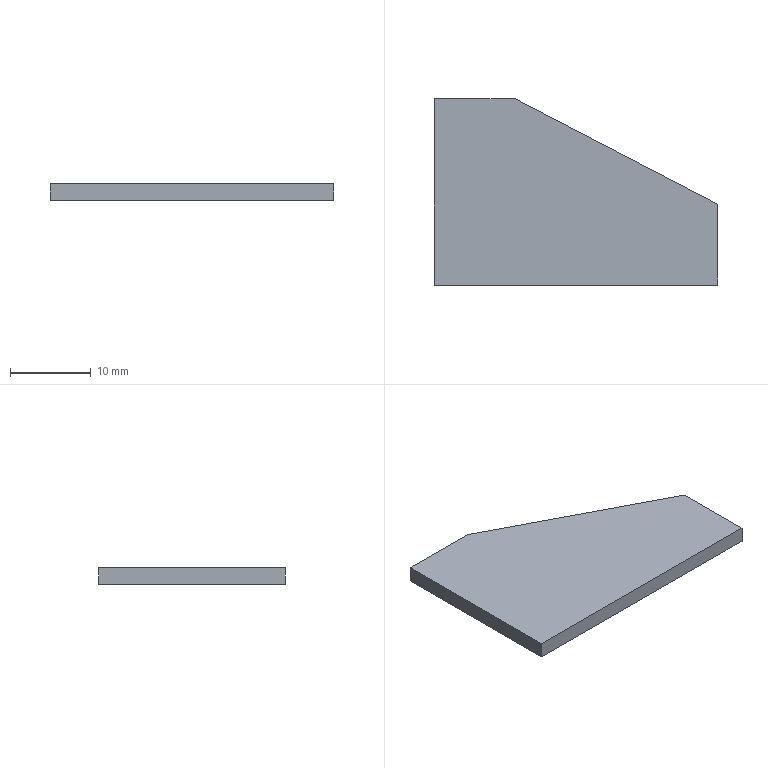Part | STEP file | Rear Base Frame-1 | 1 solid | 7 faces | box 35 x 23 x 2 mm | volume 1285 mm3 | plane 7
STEP:
#1=CARTESIAN_POINT('',(71.518,-60.079,-2.));
#2=VERTEX_POINT('',#1);
#3=CARTESIAN_POINT('',(36.518,-60.079,-2.));
#4=VERTEX_POINT('',#3);
#5=CARTESIAN_POINT('',(0.,-60.079,-2.));
#6=DIRECTION('',(-1.,0.,0.));
#7=VECTOR('',#6,1000.);
#8=LINE('',#5,#7);
#9=EDGE_CURVE('',#2,#4,#8,.T.);
#10=ORIENTED_EDGE('',*,*,#9,.T.);
#11=CARTESIAN_POINT('',(36.518,-37.079,-2.));
#12=VERTEX_POINT('',#11);
#13=CARTESIAN_POINT('',(36.518,0.,-2.));
#14=DIRECTION('',(0.,1.,0.));
#15=VECTOR('',#14,1000.);
#16=LINE('',#13,#15);
#17=EDGE_CURVE('',#4,#12,#16,.T.);
#18=ORIENTED_EDGE('',*,*,#17,.T.);
#19=CARTESIAN_POINT('',(46.518,-37.079,-2.));
#20=VERTEX_POINT('',#19);
#21=CARTESIAN_POINT('',(0.,-37.079,-2.));
#22=DIRECTION('',(1.,0.,0.));
#23=VECTOR('',#22,1000.);
#24=LINE('',#21,#23);
#25=EDGE_CURVE('',#12,#20,#24,.T.);
#26=ORIENTED_EDGE('',*,*,#25,.T.);
#27=CARTESIAN_POINT('',(71.518,-50.079,-2.));
#28=VERTEX_POINT('',#27);
#29=CARTESIAN_POINT('',(46.518,-37.079,-2.));
#30=DIRECTION('',(0.8872,-0.4614,0.));
#31=VECTOR('',#30,1000.);
#32=LINE('',#29,#31);
#33=EDGE_CURVE('',#20,#28,#32,.T.);
#34=ORIENTED_EDGE('',*,*,#33,.T.);
#35=CARTESIAN_POINT('',(71.518,0.,-2.));
#36=DIRECTION('',(0.,-1.,0.));
#37=VECTOR('',#36,1000.);
#38=LINE('',#35,#37);
#39=EDGE_CURVE('',#28,#2,#38,.T.);
#40=ORIENTED_EDGE('',*,*,#39,.T.);
#41=EDGE_LOOP('',(#10,#18,#26,#34,#40));
#42=FACE_OUTER_BOUND('',#41,.T.);
#43=CARTESIAN_POINT('',(0.,0.,-2.));
#44=DIRECTION('',(0.,0.,-1.));
#45=DIRECTION('',(-1.,0.,0.));
#46=AXIS2_PLACEMENT_3D('',#43,#44,#45);
#47=PLANE('',#46);
#48=ADVANCED_FACE('',(#42),#47,.T.);
#49=ORIENTED_EDGE('',*,*,#17,.F.);
#50=CARTESIAN_POINT('',(36.518,-60.079,0.));
#51=VERTEX_POINT('',#50);
#52=CARTESIAN_POINT('',(36.518,-60.079,-2.));
#53=DIRECTION('',(0.,0.,1.));
#54=VECTOR('',#53,1000.);
#55=LINE('',#52,#54);
#56=EDGE_CURVE('',#4,#51,#55,.T.);
#57=ORIENTED_EDGE('',*,*,#56,.T.);
#58=CARTESIAN_POINT('',(36.518,-37.079,0.));
#59=VERTEX_POINT('',#58);
#60=CARTESIAN_POINT('',(36.518,-37.079,0.));
#61=DIRECTION('',(0.,1.,0.));
#62=VECTOR('',#61,1000.);
#63=LINE('',#60,#62);
#64=EDGE_CURVE('',#51,#59,#63,.T.);
#65=ORIENTED_EDGE('',*,*,#64,.T.);
#66=CARTESIAN_POINT('',(36.518,-37.079,-2.));
#67=DIRECTION('',(0.,0.,-1.));
#68=VECTOR('',#67,1000.);
#69=LINE('',#66,#68);
#70=EDGE_CURVE('',#59,#12,#69,.T.);
#71=ORIENTED_EDGE('',*,*,#70,.T.);
#72=EDGE_LOOP('',(#49,#57,#65,#71));
#73=FACE_OUTER_BOUND('',#72,.T.);
#74=CARTESIAN_POINT('',(36.518,-37.079,-2.));
#75=DIRECTION('',(-1.,0.,0.));
#76=DIRECTION('',(0.,-1.,0.));
#77=AXIS2_PLACEMENT_3D('',#74,#75,#76);
#78=PLANE('',#77);
#79=ADVANCED_FACE('',(#73),#78,.T.);
#80=ORIENTED_EDGE('',*,*,#9,.F.);
#81=CARTESIAN_POINT('',(71.518,-60.079,0.));
#82=VERTEX_POINT('',#81);
#83=CARTESIAN_POINT('',(71.518,-60.079,-2.));
#84=DIRECTION('',(0.,0.,1.));
#85=VECTOR('',#84,1000.);
#86=LINE('',#83,#85);
#87=EDGE_CURVE('',#2,#82,#86,.T.);
#88=ORIENTED_EDGE('',*,*,#87,.T.);
#89=CARTESIAN_POINT('',(36.518,-60.079,0.));
#90=DIRECTION('',(-1.,0.,0.));
#91=VECTOR('',#90,1000.);
#92=LINE('',#89,#91);
#93=EDGE_CURVE('',#82,#51,#92,.T.);
#94=ORIENTED_EDGE('',*,*,#93,.T.);
#95=ORIENTED_EDGE('',*,*,#56,.F.);
#96=EDGE_LOOP('',(#80,#88,#94,#95));
#97=FACE_OUTER_BOUND('',#96,.T.);
#98=CARTESIAN_POINT('',(36.518,-60.079,-2.));
#99=DIRECTION('',(0.,-1.,0.));
#100=DIRECTION('',(0.,0.,-1.));
#101=AXIS2_PLACEMENT_3D('',#98,#99,#100);
#102=PLANE('',#101);
#103=ADVANCED_FACE('',(#97),#102,.T.);
#104=ORIENTED_EDGE('',*,*,#39,.F.);
#105=CARTESIAN_POINT('',(71.518,-50.079,0.));
#106=VERTEX_POINT('',#105);
#107=CARTESIAN_POINT('',(71.518,-50.079,-2.));
#108=DIRECTION('',(0.,0.,1.));
#109=VECTOR('',#108,1000.);
#110=LINE('',#107,#109);
#111=EDGE_CURVE('',#28,#106,#110,.T.);
#112=ORIENTED_EDGE('',*,*,#111,.T.);
#113=CARTESIAN_POINT('',(71.518,-50.079,0.));
#114=DIRECTION('',(0.,-1.,0.));
#115=VECTOR('',#114,1000.);
#116=LINE('',#113,#115);
#117=EDGE_CURVE('',#106,#82,#116,.T.);
#118=ORIENTED_EDGE('',*,*,#117,.T.);
#119=ORIENTED_EDGE('',*,*,#87,.F.);
#120=EDGE_LOOP('',(#104,#112,#118,#119));
#121=FACE_OUTER_BOUND('',#120,.T.);
#122=CARTESIAN_POINT('',(71.518,-50.079,-2.));
#123=DIRECTION('',(1.,0.,0.));
#124=DIRECTION('',(0.,0.,-1.));
#125=AXIS2_PLACEMENT_3D('',#122,#123,#124);
#126=PLANE('',#125);
#127=ADVANCED_FACE('',(#121),#126,.T.);
#128=ORIENTED_EDGE('',*,*,#33,.F.);
#129=CARTESIAN_POINT('',(46.518,-37.079,0.));
#130=VERTEX_POINT('',#129);
#131=CARTESIAN_POINT('',(46.518,-37.079,-2.));
#132=DIRECTION('',(0.,0.,1.));
#133=VECTOR('',#132,1000.);
#134=LINE('',#131,#133);
#135=EDGE_CURVE('',#20,#130,#134,.T.);
#136=ORIENTED_EDGE('',*,*,#135,.T.);
#137=CARTESIAN_POINT('',(46.518,-37.079,0.));
#138=DIRECTION('',(0.8872,-0.4614,0.));
#139=VECTOR('',#138,1000.);
#140=LINE('',#137,#139);
#141=EDGE_CURVE('',#130,#106,#140,.T.);
#142=ORIENTED_EDGE('',*,*,#141,.T.);
#143=ORIENTED_EDGE('',*,*,#111,.F.);
#144=EDGE_LOOP('',(#128,#136,#142,#143));
#145=FACE_OUTER_BOUND('',#144,.T.);
#146=CARTESIAN_POINT('',(46.518,-37.079,-2.));
#147=DIRECTION('',(0.4614,0.8872,0.));
#148=DIRECTION('',(-0.8872,0.4614,0.));
#149=AXIS2_PLACEMENT_3D('',#146,#147,#148);
#150=PLANE('',#149);
#151=ADVANCED_FACE('',(#145),#150,.T.);
#152=ORIENTED_EDGE('',*,*,#25,.F.);
#153=ORIENTED_EDGE('',*,*,#70,.F.);
#154=CARTESIAN_POINT('',(36.518,-37.079,0.));
#155=DIRECTION('',(1.,0.,0.));
#156=VECTOR('',#155,1000.);
#157=LINE('',#154,#156);
#158=EDGE_CURVE('',#59,#130,#157,.T.);
#159=ORIENTED_EDGE('',*,*,#158,.T.);
#160=ORIENTED_EDGE('',*,*,#135,.F.);
#161=EDGE_LOOP('',(#152,#153,#159,#160));
#162=FACE_OUTER_BOUND('',#161,.T.);
#163=CARTESIAN_POINT('',(36.518,-37.079,-2.));
#164=DIRECTION('',(0.,1.,0.));
#165=DIRECTION('',(0.,0.,1.));
#166=AXIS2_PLACEMENT_3D('',#163,#164,#165);
#167=PLANE('',#166);
#168=ADVANCED_FACE('',(#162),#167,.T.);
#169=ORIENTED_EDGE('',*,*,#64,.F.);
#170=ORIENTED_EDGE('',*,*,#93,.F.);
#171=ORIENTED_EDGE('',*,*,#117,.F.);
#172=ORIENTED_EDGE('',*,*,#141,.F.);
#173=ORIENTED_EDGE('',*,*,#158,.F.);
#174=EDGE_LOOP('',(#169,#170,#171,#172,#173));
#175=FACE_OUTER_BOUND('',#174,.T.);
#176=CARTESIAN_POINT('',(0.,0.,0.));
#177=DIRECTION('',(0.,0.,-1.));
#178=DIRECTION('',(-1.,0.,0.));
#179=AXIS2_PLACEMENT_3D('',#176,#177,#178);
#180=PLANE('',#179);
#181=ADVANCED_FACE('',(#175),#180,.F.);
#182=CLOSED_SHELL('',(#48,#79,#103,#127,#151,#168,#181));
#183=MANIFOLD_SOLID_BREP('',#182);
#184=CARTESIAN_POINT('',(0.,0.,0.));
#185=DIRECTION('',(0.,0.,1.));
#186=DIRECTION('',(1.,0.,0.));
#187=AXIS2_PLACEMENT_3D('',#184,#185,#186);
#188=(LENGTH_UNIT()NAMED_UNIT(*)SI_UNIT(.MILLI.,.METRE.));
#189=UNCERTAINTY_MEASURE_WITH_UNIT(LENGTH_MEASURE(0.00001),#188,'','');
#190=(NAMED_UNIT(*)PLANE_ANGLE_UNIT()SI_UNIT($,.RADIAN.));
#191=(NAMED_UNIT(*)SI_UNIT($,.STERADIAN.)SOLID_ANGLE_UNIT());
#192=(GEOMETRIC_REPRESENTATION_CONTEXT(3)GLOBAL_UNCERTAINTY_ASSIGNED_CONTEXT((#189))GLOBAL_UNIT_ASSIGNED_CONTEXT((#188,#190,#191))REPRESENTATION_CONTEXT('',''));
#193=ADVANCED_BREP_SHAPE_REPRESENTATION('',(#183,#187),#192);